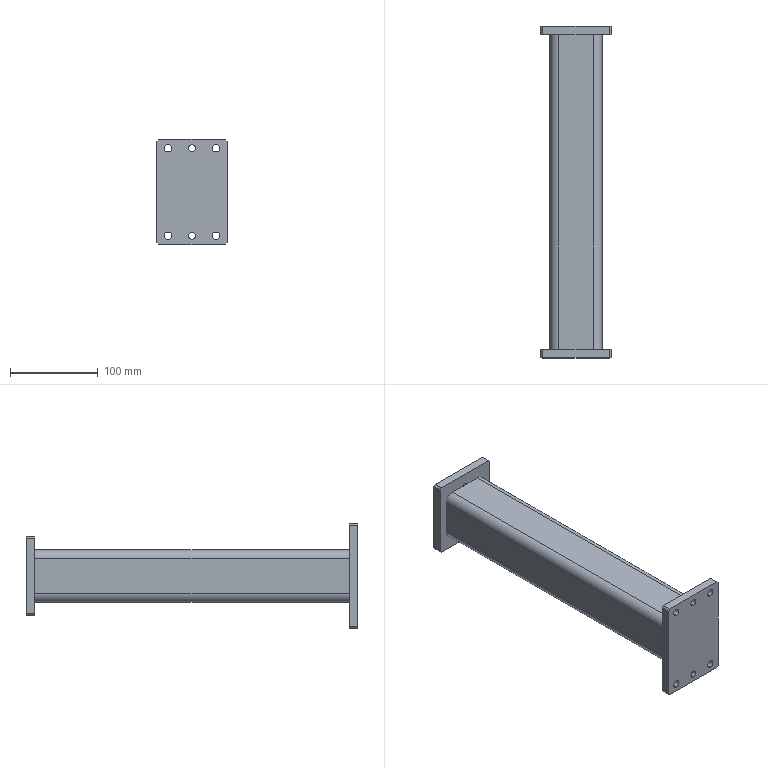Part | SolidWorks | features HoleWzd 4, Chamfer 2, ICE 2, WeldMemberFeat 1, WeldmentFeature 1 | 3 solids | 56 faces | box 80 x 379 x 120 mm | volume 535710 mm3 | plane 30 | cylinder 26 | commonest cylinder face diameters 8.6 x8 5 x6 8 x4 10 x4 20 x4